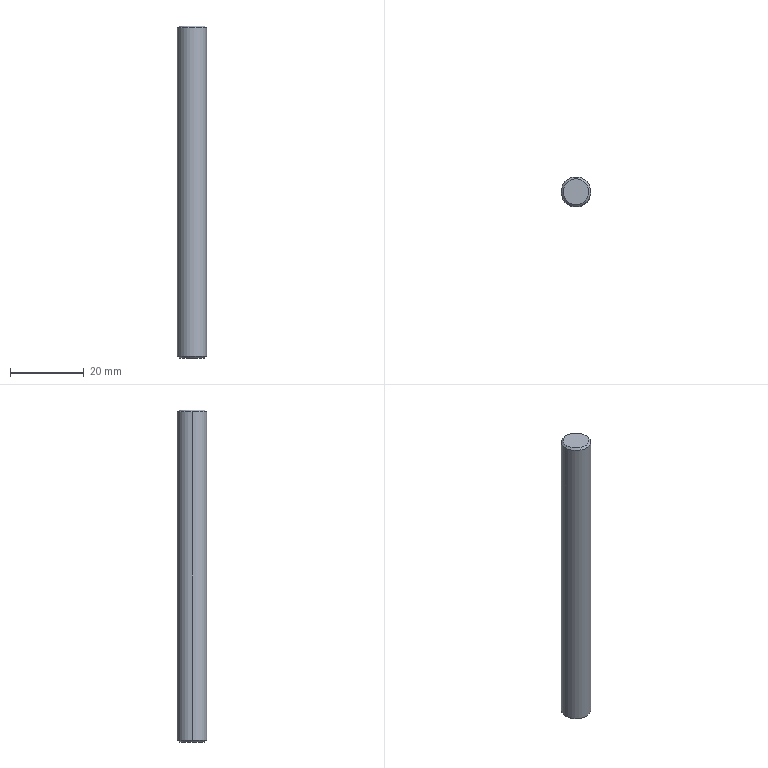Part | STEP file | BCC3 H14_5 | 1 solid | 8 faces | box 8 x 8 x 90 mm | volume 4518 mm3 | cone 4 | cylinder 2 | plane 2 | commonest cylinder face diameters 8 x2
STEP:
#1=CARTESIAN_POINT('',(0.,0.,0.));
#2=DIRECTION('',(0.,0.,1.));
#3=DIRECTION('',(1.,0.,0.));
#4=AXIS2_PLACEMENT_3D('',#1,#2,#3);
#5=CARTESIAN_POINT('',(3.5,0.,45.));
#6=VERTEX_POINT('',#5);
#7=CARTESIAN_POINT('',(-3.5,0.,45.));
#8=VERTEX_POINT('',#7);
#9=CARTESIAN_POINT('',(0.,0.,45.));
#10=DIRECTION('',(0.,0.,1.));
#11=DIRECTION('',(1.,0.,0.));
#12=AXIS2_PLACEMENT_3D('',#9,#10,#11);
#13=CIRCLE('',#12,3.5);
#14=CARTESIAN_POINT('',(0.,0.,45.));
#15=DIRECTION('',(0.,0.,-1.));
#16=DIRECTION('',(-1.,0.,0.));
#17=AXIS2_PLACEMENT_3D('',#14,#15,#16);
#18=CONICAL_SURFACE('',#17,3.5,0.7854);
#19=CARTESIAN_POINT('',(3.142,0.));
#20=DIRECTION('',(-1.,0.));
#21=VECTOR('',#20,1.);
#22=LINE('',#19,#21);
#23=(GEOMETRIC_REPRESENTATION_CONTEXT(2)PARAMETRIC_REPRESENTATION_CONTEXT()REPRESENTATION_CONTEXT('',''));
#24=DEFINITIONAL_REPRESENTATION('',(#22),#23);
#25=PCURVE('',#18,#24);
#26=CARTESIAN_POINT('',(0.,0.,45.));
#27=DIRECTION('',(0.,0.,1.));
#28=DIRECTION('',(1.,0.,0.));
#29=AXIS2_PLACEMENT_3D('',#26,#27,#28);
#30=PLANE('',#29);
#31=CARTESIAN_POINT('',(0.,0.));
#32=DIRECTION('',(1.,0.));
#33=AXIS2_PLACEMENT_2D('',#31,#32);
#34=CIRCLE('',#33,3.5);
#35=(GEOMETRIC_REPRESENTATION_CONTEXT(2)PARAMETRIC_REPRESENTATION_CONTEXT()REPRESENTATION_CONTEXT('',''));
#36=DEFINITIONAL_REPRESENTATION('',(#34),#35);
#37=PCURVE('',#30,#36);
#38=SURFACE_CURVE('',#13,(#25,#37),.PCURVE_S1.);
#39=EDGE_CURVE('',#6,#8,#38,.T.);
#40=ORIENTED_EDGE('',*,*,#39,.F.);
#41=CARTESIAN_POINT('',(4.,0.,44.5));
#42=VERTEX_POINT('',#41);
#43=CARTESIAN_POINT('',(3.5,0.,45.));
#44=DIRECTION('',(0.7071,0.,-0.7071));
#45=VECTOR('',#44,1.);
#46=LINE('',#43,#45);
#47=CARTESIAN_POINT('',(3.142,0.));
#48=DIRECTION('',(0.,1.));
#49=VECTOR('',#48,1.);
#50=LINE('',#47,#49);
#51=(GEOMETRIC_REPRESENTATION_CONTEXT(2)PARAMETRIC_REPRESENTATION_CONTEXT()REPRESENTATION_CONTEXT('',''));
#52=DEFINITIONAL_REPRESENTATION('',(#50),#51);
#53=PCURVE('',#18,#52);
#54=CARTESIAN_POINT('',(0.,0.,45.));
#55=DIRECTION('',(0.,0.,-1.));
#56=DIRECTION('',(-1.,0.,0.));
#57=AXIS2_PLACEMENT_3D('',#54,#55,#56);
#58=CONICAL_SURFACE('',#57,3.5,0.7854);
#59=CARTESIAN_POINT('',(3.142,0.));
#60=DIRECTION('',(0.,1.));
#61=VECTOR('',#60,1.);
#62=LINE('',#59,#61);
#63=(GEOMETRIC_REPRESENTATION_CONTEXT(2)PARAMETRIC_REPRESENTATION_CONTEXT()REPRESENTATION_CONTEXT('',''));
#64=DEFINITIONAL_REPRESENTATION('',(#62),#63);
#65=PCURVE('',#58,#64);
#66=SURFACE_CURVE('',#46,(#53,#65),.PCURVE_S1.);
#67=EDGE_CURVE('',#6,#42,#66,.T.);
#68=ORIENTED_EDGE('',*,*,#67,.T.);
#69=CARTESIAN_POINT('',(-4.,0.,44.5));
#70=VERTEX_POINT('',#69);
#71=CARTESIAN_POINT('',(0.,0.,44.5));
#72=DIRECTION('',(0.,0.,-1.));
#73=DIRECTION('',(1.,0.,0.));
#74=AXIS2_PLACEMENT_3D('',#71,#72,#73);
#75=CIRCLE('',#74,4.);
#76=CARTESIAN_POINT('',(-3.142,0.5));
#77=DIRECTION('',(1.,0.));
#78=VECTOR('',#77,1.);
#79=LINE('',#76,#78);
#80=(GEOMETRIC_REPRESENTATION_CONTEXT(2)PARAMETRIC_REPRESENTATION_CONTEXT()REPRESENTATION_CONTEXT('',''));
#81=DEFINITIONAL_REPRESENTATION('',(#79),#80);
#82=PCURVE('',#18,#81);
#83=CARTESIAN_POINT('',(0.,0.,45.));
#84=DIRECTION('',(0.,0.,-1.));
#85=DIRECTION('',(-1.,0.,0.));
#86=AXIS2_PLACEMENT_3D('',#83,#84,#85);
#87=CYLINDRICAL_SURFACE('',#86,4.);
#88=CARTESIAN_POINT('',(-3.142,0.5));
#89=DIRECTION('',(1.,0.));
#90=VECTOR('',#89,1.);
#91=LINE('',#88,#90);
#92=(GEOMETRIC_REPRESENTATION_CONTEXT(2)PARAMETRIC_REPRESENTATION_CONTEXT()REPRESENTATION_CONTEXT('',''));
#93=DEFINITIONAL_REPRESENTATION('',(#91),#92);
#94=PCURVE('',#87,#93);
#95=SURFACE_CURVE('',#75,(#82,#94),.PCURVE_S1.);
#96=EDGE_CURVE('',#70,#42,#95,.T.);
#97=ORIENTED_EDGE('',*,*,#96,.F.);
#98=CARTESIAN_POINT('',(-3.5,0.,45.));
#99=DIRECTION('',(-0.7071,0.,-0.7071));
#100=VECTOR('',#99,1.);
#101=LINE('',#98,#100);
#102=CARTESIAN_POINT('',(0.,0.));
#103=DIRECTION('',(0.,1.));
#104=VECTOR('',#103,1.);
#105=LINE('',#102,#104);
#106=(GEOMETRIC_REPRESENTATION_CONTEXT(2)PARAMETRIC_REPRESENTATION_CONTEXT()REPRESENTATION_CONTEXT('',''));
#107=DEFINITIONAL_REPRESENTATION('',(#105),#106);
#108=PCURVE('',#18,#107);
#109=CARTESIAN_POINT('',(6.283,0.));
#110=DIRECTION('',(0.,1.));
#111=VECTOR('',#110,1.);
#112=LINE('',#109,#111);
#113=(GEOMETRIC_REPRESENTATION_CONTEXT(2)PARAMETRIC_REPRESENTATION_CONTEXT()REPRESENTATION_CONTEXT('',''));
#114=DEFINITIONAL_REPRESENTATION('',(#112),#113);
#115=PCURVE('',#58,#114);
#116=SURFACE_CURVE('',#101,(#108,#115),.PCURVE_S1.);
#117=EDGE_CURVE('',#8,#70,#116,.T.);
#118=ORIENTED_EDGE('',*,*,#117,.F.);
#119=EDGE_LOOP('',(#40,#68,#97,#118));
#120=FACE_BOUND('',#119,.T.);
#121=ADVANCED_FACE('',(#120),#18,.T.);
#122=CARTESIAN_POINT('',(-3.5,0.,-45.));
#123=VERTEX_POINT('',#122);
#124=CARTESIAN_POINT('',(3.5,0.,-45.));
#125=VERTEX_POINT('',#124);
#126=CARTESIAN_POINT('',(0.,0.,-45.));
#127=DIRECTION('',(0.,0.,-1.));
#128=DIRECTION('',(1.,0.,0.));
#129=AXIS2_PLACEMENT_3D('',#126,#127,#128);
#130=CIRCLE('',#129,3.5);
#131=CARTESIAN_POINT('',(0.,0.,-44.5));
#132=DIRECTION('',(0.,0.,1.));
#133=DIRECTION('',(1.,0.,0.));
#134=AXIS2_PLACEMENT_3D('',#131,#132,#133);
#135=CONICAL_SURFACE('',#134,4.,0.7854);
#136=CARTESIAN_POINT('',(6.283,-0.5));
#137=DIRECTION('',(-1.,0.));
#138=VECTOR('',#137,1.);
#139=LINE('',#136,#138);
#140=(GEOMETRIC_REPRESENTATION_CONTEXT(2)PARAMETRIC_REPRESENTATION_CONTEXT()REPRESENTATION_CONTEXT('',''));
#141=DEFINITIONAL_REPRESENTATION('',(#139),#140);
#142=PCURVE('',#135,#141);
#143=CARTESIAN_POINT('',(0.,0.,-45.));
#144=DIRECTION('',(0.,0.,1.));
#145=DIRECTION('',(1.,0.,0.));
#146=AXIS2_PLACEMENT_3D('',#143,#144,#145);
#147=PLANE('',#146);
#148=CARTESIAN_POINT('',(3.5,0.));
#149=CARTESIAN_POINT('',(3.5,-6.062));
#150=CARTESIAN_POINT('',(-1.75,-3.031));
#151=CARTESIAN_POINT('',(-7.,0.));
#152=CARTESIAN_POINT('',(-1.75,3.031));
#153=CARTESIAN_POINT('',(3.5,6.062));
#154=CARTESIAN_POINT('',(3.5,0.));
#155=(BOUNDED_CURVE()B_SPLINE_CURVE(2,(#148,#149,#150,#151,#152,#153,#154),.UNSPECIFIED.,.T.,.F.)B_SPLINE_CURVE_WITH_KNOTS((1,2,2,2,2,1),(-2.094,0.,2.094,4.189,6.283,8.378),.UNSPECIFIED.)CURVE()GEOMETRIC_REPRESENTATION_ITEM()RATIONAL_B_SPLINE_CURVE((1.,0.5,1.,0.5,1.,0.5,1.))REPRESENTATION_ITEM(''));
#156=(GEOMETRIC_REPRESENTATION_CONTEXT(2)PARAMETRIC_REPRESENTATION_CONTEXT()REPRESENTATION_CONTEXT('',''));
#157=DEFINITIONAL_REPRESENTATION('',(#155),#156);
#158=PCURVE('',#147,#157);
#159=SURFACE_CURVE('',#130,(#142,#158),.PCURVE_S1.);
#160=EDGE_CURVE('',#123,#125,#159,.T.);
#161=ORIENTED_EDGE('',*,*,#160,.F.);
#162=CARTESIAN_POINT('',(-4.,0.,-44.5));
#163=VERTEX_POINT('',#162);
#164=CARTESIAN_POINT('',(-4.,0.,-44.5));
#165=DIRECTION('',(-0.7071,0.,0.7071));
#166=VECTOR('',#165,1.);
#167=LINE('',#164,#166);
#168=CARTESIAN_POINT('',(3.142,0.));
#169=DIRECTION('',(0.,1.));
#170=VECTOR('',#169,1.);
#171=LINE('',#168,#170);
#172=(GEOMETRIC_REPRESENTATION_CONTEXT(2)PARAMETRIC_REPRESENTATION_CONTEXT()REPRESENTATION_CONTEXT('',''));
#173=DEFINITIONAL_REPRESENTATION('',(#171),#172);
#174=PCURVE('',#135,#173);
#175=CARTESIAN_POINT('',(0.,0.,-44.5));
#176=DIRECTION('',(0.,0.,1.));
#177=DIRECTION('',(1.,0.,0.));
#178=AXIS2_PLACEMENT_3D('',#175,#176,#177);
#179=CONICAL_SURFACE('',#178,4.,0.7854);
#180=CARTESIAN_POINT('',(3.142,0.));
#181=DIRECTION('',(0.,1.));
#182=VECTOR('',#181,1.);
#183=LINE('',#180,#182);
#184=(GEOMETRIC_REPRESENTATION_CONTEXT(2)PARAMETRIC_REPRESENTATION_CONTEXT()REPRESENTATION_CONTEXT('',''));
#185=DEFINITIONAL_REPRESENTATION('',(#183),#184);
#186=PCURVE('',#179,#185);
#187=SURFACE_CURVE('',#167,(#174,#186),.PCURVE_S1.);
#188=EDGE_CURVE('',#123,#163,#187,.T.);
#189=ORIENTED_EDGE('',*,*,#188,.T.);
#190=CARTESIAN_POINT('',(4.,0.,-44.5));
#191=VERTEX_POINT('',#190);
#192=CARTESIAN_POINT('',(0.,0.,-44.5));
#193=DIRECTION('',(0.,0.,1.));
#194=DIRECTION('',(1.,0.,0.));
#195=AXIS2_PLACEMENT_3D('',#192,#193,#194);
#196=CIRCLE('',#195,4.);
#197=CARTESIAN_POINT('',(0.,0.));
#198=DIRECTION('',(1.,0.));
#199=VECTOR('',#198,1.);
#200=LINE('',#197,#199);
#201=(GEOMETRIC_REPRESENTATION_CONTEXT(2)PARAMETRIC_REPRESENTATION_CONTEXT()REPRESENTATION_CONTEXT('',''));
#202=DEFINITIONAL_REPRESENTATION('',(#200),#201);
#203=PCURVE('',#135,#202);
#204=CARTESIAN_POINT('',(3.142,89.5));
#205=DIRECTION('',(-1.,0.));
#206=VECTOR('',#205,1.);
#207=LINE('',#204,#206);
#208=(GEOMETRIC_REPRESENTATION_CONTEXT(2)PARAMETRIC_REPRESENTATION_CONTEXT()REPRESENTATION_CONTEXT('',''));
#209=DEFINITIONAL_REPRESENTATION('',(#207),#208);
#210=PCURVE('',#87,#209);
#211=SURFACE_CURVE('',#196,(#203,#210),.PCURVE_S1.);
#212=EDGE_CURVE('',#191,#163,#211,.T.);
#213=ORIENTED_EDGE('',*,*,#212,.F.);
#214=CARTESIAN_POINT('',(4.,0.,-44.5));
#215=DIRECTION('',(0.7071,0.,0.7071));
#216=VECTOR('',#215,1.);
#217=LINE('',#214,#216);
#218=CARTESIAN_POINT('',(0.,0.));
#219=DIRECTION('',(0.,1.));
#220=VECTOR('',#219,1.);
#221=LINE('',#218,#220);
#222=(GEOMETRIC_REPRESENTATION_CONTEXT(2)PARAMETRIC_REPRESENTATION_CONTEXT()REPRESENTATION_CONTEXT('',''));
#223=DEFINITIONAL_REPRESENTATION('',(#221),#222);
#224=PCURVE('',#135,#223);
#225=CARTESIAN_POINT('',(6.283,0.));
#226=DIRECTION('',(0.,1.));
#227=VECTOR('',#226,1.);
#228=LINE('',#225,#227);
#229=(GEOMETRIC_REPRESENTATION_CONTEXT(2)PARAMETRIC_REPRESENTATION_CONTEXT()REPRESENTATION_CONTEXT('',''));
#230=DEFINITIONAL_REPRESENTATION('',(#228),#229);
#231=PCURVE('',#179,#230);
#232=SURFACE_CURVE('',#217,(#224,#231),.PCURVE_S1.);
#233=EDGE_CURVE('',#125,#191,#232,.T.);
#234=ORIENTED_EDGE('',*,*,#233,.F.);
#235=EDGE_LOOP('',(#161,#189,#213,#234));
#236=FACE_BOUND('',#235,.T.);
#237=ADVANCED_FACE('',(#236),#135,.T.);
#238=ORIENTED_EDGE('',*,*,#96,.T.);
#239=CARTESIAN_POINT('',(4.,0.,45.));
#240=DIRECTION('',(0.,0.,-1.));
#241=VECTOR('',#240,1.);
#242=LINE('',#239,#241);
#243=CARTESIAN_POINT('',(3.142,0.));
#244=DIRECTION('',(0.,1.));
#245=VECTOR('',#244,1.);
#246=LINE('',#243,#245);
#247=(GEOMETRIC_REPRESENTATION_CONTEXT(2)PARAMETRIC_REPRESENTATION_CONTEXT()REPRESENTATION_CONTEXT('',''));
#248=DEFINITIONAL_REPRESENTATION('',(#246),#247);
#249=PCURVE('',#87,#248);
#250=CARTESIAN_POINT('',(0.,0.,45.));
#251=DIRECTION('',(0.,0.,-1.));
#252=DIRECTION('',(-1.,0.,0.));
#253=AXIS2_PLACEMENT_3D('',#250,#251,#252);
#254=CYLINDRICAL_SURFACE('',#253,4.);
#255=CARTESIAN_POINT('',(3.142,0.));
#256=DIRECTION('',(0.,1.));
#257=VECTOR('',#256,1.);
#258=LINE('',#255,#257);
#259=(GEOMETRIC_REPRESENTATION_CONTEXT(2)PARAMETRIC_REPRESENTATION_CONTEXT()REPRESENTATION_CONTEXT('',''));
#260=DEFINITIONAL_REPRESENTATION('',(#258),#259);
#261=PCURVE('',#254,#260);
#262=SURFACE_CURVE('',#242,(#249,#261),.PCURVE_S1.);
#263=EDGE_CURVE('',#42,#191,#262,.T.);
#264=ORIENTED_EDGE('',*,*,#263,.T.);
#265=ORIENTED_EDGE('',*,*,#212,.T.);
#266=CARTESIAN_POINT('',(-4.,0.,45.));
#267=DIRECTION('',(0.,0.,-1.));
#268=VECTOR('',#267,1.);
#269=LINE('',#266,#268);
#270=CARTESIAN_POINT('',(0.,0.));
#271=DIRECTION('',(0.,1.));
#272=VECTOR('',#271,1.);
#273=LINE('',#270,#272);
#274=(GEOMETRIC_REPRESENTATION_CONTEXT(2)PARAMETRIC_REPRESENTATION_CONTEXT()REPRESENTATION_CONTEXT('',''));
#275=DEFINITIONAL_REPRESENTATION('',(#273),#274);
#276=PCURVE('',#87,#275);
#277=CARTESIAN_POINT('',(6.283,0.));
#278=DIRECTION('',(0.,1.));
#279=VECTOR('',#278,1.);
#280=LINE('',#277,#279);
#281=(GEOMETRIC_REPRESENTATION_CONTEXT(2)PARAMETRIC_REPRESENTATION_CONTEXT()REPRESENTATION_CONTEXT('',''));
#282=DEFINITIONAL_REPRESENTATION('',(#280),#281);
#283=PCURVE('',#254,#282);
#284=SURFACE_CURVE('',#269,(#276,#283),.PCURVE_S1.);
#285=EDGE_CURVE('',#70,#163,#284,.T.);
#286=ORIENTED_EDGE('',*,*,#285,.F.);
#287=EDGE_LOOP('',(#238,#264,#265,#286));
#288=FACE_BOUND('',#287,.T.);
#289=ADVANCED_FACE('',(#288),#87,.T.);
#290=ORIENTED_EDGE('',*,*,#263,.F.);
#291=CARTESIAN_POINT('',(0.,0.,44.5));
#292=DIRECTION('',(0.,0.,-1.));
#293=DIRECTION('',(1.,0.,0.));
#294=AXIS2_PLACEMENT_3D('',#291,#292,#293);
#295=CIRCLE('',#294,4.);
#296=CARTESIAN_POINT('',(3.142,0.5));
#297=DIRECTION('',(1.,0.));
#298=VECTOR('',#297,1.);
#299=LINE('',#296,#298);
#300=(GEOMETRIC_REPRESENTATION_CONTEXT(2)PARAMETRIC_REPRESENTATION_CONTEXT()REPRESENTATION_CONTEXT('',''));
#301=DEFINITIONAL_REPRESENTATION('',(#299),#300);
#302=PCURVE('',#254,#301);
#303=CARTESIAN_POINT('',(3.142,0.5));
#304=DIRECTION('',(1.,0.));
#305=VECTOR('',#304,1.);
#306=LINE('',#303,#305);
#307=(GEOMETRIC_REPRESENTATION_CONTEXT(2)PARAMETRIC_REPRESENTATION_CONTEXT()REPRESENTATION_CONTEXT('',''));
#308=DEFINITIONAL_REPRESENTATION('',(#306),#307);
#309=PCURVE('',#58,#308);
#310=SURFACE_CURVE('',#295,(#302,#309),.PCURVE_S1.);
#311=EDGE_CURVE('',#42,#70,#310,.T.);
#312=ORIENTED_EDGE('',*,*,#311,.T.);
#313=ORIENTED_EDGE('',*,*,#285,.T.);
#314=CARTESIAN_POINT('',(0.,0.,-44.5));
#315=DIRECTION('',(0.,0.,1.));
#316=DIRECTION('',(1.,0.,0.));
#317=AXIS2_PLACEMENT_3D('',#314,#315,#316);
#318=CIRCLE('',#317,4.);
#319=CARTESIAN_POINT('',(9.425,89.5));
#320=DIRECTION('',(-1.,0.));
#321=VECTOR('',#320,1.);
#322=LINE('',#319,#321);
#323=(GEOMETRIC_REPRESENTATION_CONTEXT(2)PARAMETRIC_REPRESENTATION_CONTEXT()REPRESENTATION_CONTEXT('',''));
#324=DEFINITIONAL_REPRESENTATION('',(#322),#323);
#325=PCURVE('',#254,#324);
#326=CARTESIAN_POINT('',(0.,0.));
#327=DIRECTION('',(1.,0.));
#328=VECTOR('',#327,1.);
#329=LINE('',#326,#328);
#330=(GEOMETRIC_REPRESENTATION_CONTEXT(2)PARAMETRIC_REPRESENTATION_CONTEXT()REPRESENTATION_CONTEXT('',''));
#331=DEFINITIONAL_REPRESENTATION('',(#329),#330);
#332=PCURVE('',#179,#331);
#333=SURFACE_CURVE('',#318,(#325,#332),.PCURVE_S1.);
#334=EDGE_CURVE('',#163,#191,#333,.T.);
#335=ORIENTED_EDGE('',*,*,#334,.T.);
#336=EDGE_LOOP('',(#290,#312,#313,#335));
#337=FACE_BOUND('',#336,.T.);
#338=ADVANCED_FACE('',(#337),#254,.T.);
#339=CARTESIAN_POINT('',(0.,0.,45.));
#340=DIRECTION('',(0.,0.,1.));
#341=DIRECTION('',(1.,0.,0.));
#342=AXIS2_PLACEMENT_3D('',#339,#340,#341);
#343=CIRCLE('',#342,3.5);
#344=CARTESIAN_POINT('',(0.,0.));
#345=DIRECTION('',(1.,0.));
#346=AXIS2_PLACEMENT_2D('',#344,#345);
#347=CIRCLE('',#346,3.5);
#348=(GEOMETRIC_REPRESENTATION_CONTEXT(2)PARAMETRIC_REPRESENTATION_CONTEXT()REPRESENTATION_CONTEXT('',''));
#349=DEFINITIONAL_REPRESENTATION('',(#347),#348);
#350=PCURVE('',#30,#349);
#351=CARTESIAN_POINT('',(9.425,0.));
#352=DIRECTION('',(-1.,0.));
#353=VECTOR('',#352,1.);
#354=LINE('',#351,#353);
#355=(GEOMETRIC_REPRESENTATION_CONTEXT(2)PARAMETRIC_REPRESENTATION_CONTEXT()REPRESENTATION_CONTEXT('',''));
#356=DEFINITIONAL_REPRESENTATION('',(#354),#355);
#357=PCURVE('',#58,#356);
#358=SURFACE_CURVE('',#343,(#350,#357),.PCURVE_S1.);
#359=EDGE_CURVE('',#8,#6,#358,.T.);
#360=ORIENTED_EDGE('',*,*,#359,.T.);
#361=ORIENTED_EDGE('',*,*,#39,.T.);
#362=EDGE_LOOP('',(#360,#361));
#363=FACE_BOUND('',#362,.T.);
#364=ADVANCED_FACE('',(#363),#30,.T.);
#365=CARTESIAN_POINT('',(0.,0.,-45.));
#366=DIRECTION('',(0.,0.,-1.));
#367=DIRECTION('',(1.,0.,0.));
#368=AXIS2_PLACEMENT_3D('',#365,#366,#367);
#369=CIRCLE('',#368,3.5);
#370=CARTESIAN_POINT('',(3.5,0.));
#371=CARTESIAN_POINT('',(3.5,-6.062));
#372=CARTESIAN_POINT('',(-1.75,-3.031));
#373=CARTESIAN_POINT('',(-7.,0.));
#374=CARTESIAN_POINT('',(-1.75,3.031));
#375=CARTESIAN_POINT('',(3.5,6.062));
#376=CARTESIAN_POINT('',(3.5,0.));
#377=(BOUNDED_CURVE()B_SPLINE_CURVE(2,(#370,#371,#372,#373,#374,#375,#376),.UNSPECIFIED.,.T.,.F.)B_SPLINE_CURVE_WITH_KNOTS((1,2,2,2,2,1),(-2.094,0.,2.094,4.189,6.283,8.378),.UNSPECIFIED.)CURVE()GEOMETRIC_REPRESENTATION_ITEM()RATIONAL_B_SPLINE_CURVE((1.,0.5,1.,0.5,1.,0.5,1.))REPRESENTATION_ITEM(''));
#378=(GEOMETRIC_REPRESENTATION_CONTEXT(2)PARAMETRIC_REPRESENTATION_CONTEXT()REPRESENTATION_CONTEXT('',''));
#379=DEFINITIONAL_REPRESENTATION('',(#377),#378);
#380=PCURVE('',#147,#379);
#381=CARTESIAN_POINT('',(6.283,-0.5));
#382=DIRECTION('',(-1.,0.));
#383=VECTOR('',#382,1.);
#384=LINE('',#381,#383);
#385=(GEOMETRIC_REPRESENTATION_CONTEXT(2)PARAMETRIC_REPRESENTATION_CONTEXT()REPRESENTATION_CONTEXT('',''));
#386=DEFINITIONAL_REPRESENTATION('',(#384),#385);
#387=PCURVE('',#179,#386);
#388=SURFACE_CURVE('',#369,(#380,#387),.PCURVE_S1.);
#389=EDGE_CURVE('',#125,#123,#388,.T.);
#390=ORIENTED_EDGE('',*,*,#389,.T.);
#391=ORIENTED_EDGE('',*,*,#160,.T.);
#392=EDGE_LOOP('',(#390,#391));
#393=FACE_BOUND('',#392,.T.);
#394=ADVANCED_FACE('',(#393),#147,.F.);
#395=ORIENTED_EDGE('',*,*,#188,.F.);
#396=ORIENTED_EDGE('',*,*,#389,.F.);
#397=ORIENTED_EDGE('',*,*,#233,.T.);
#398=ORIENTED_EDGE('',*,*,#334,.F.);
#399=EDGE_LOOP('',(#395,#396,#397,#398));
#400=FACE_BOUND('',#399,.T.);
#401=ADVANCED_FACE('',(#400),#179,.T.);
#402=ORIENTED_EDGE('',*,*,#67,.F.);
#403=ORIENTED_EDGE('',*,*,#359,.F.);
#404=ORIENTED_EDGE('',*,*,#117,.T.);
#405=ORIENTED_EDGE('',*,*,#311,.F.);
#406=EDGE_LOOP('',(#402,#403,#404,#405));
#407=FACE_BOUND('',#406,.T.);
#408=ADVANCED_FACE('',(#407),#58,.T.);
#409=CLOSED_SHELL('',(#121,#237,#289,#338,#364,#394,#401,#408));
#410=MANIFOLD_SOLID_BREP('',#409);
#411=(LENGTH_UNIT()NAMED_UNIT(*)SI_UNIT(.MILLI.,.METRE.));
#412=UNCERTAINTY_MEASURE_WITH_UNIT(LENGTH_MEASURE(0.0000001),#411,'','');
#413=(NAMED_UNIT(*)PLANE_ANGLE_UNIT()SI_UNIT($,.RADIAN.));
#414=(NAMED_UNIT(*)SI_UNIT($,.STERADIAN.)SOLID_ANGLE_UNIT());
#415=(GEOMETRIC_REPRESENTATION_CONTEXT(3)GLOBAL_UNCERTAINTY_ASSIGNED_CONTEXT((#412))GLOBAL_UNIT_ASSIGNED_CONTEXT((#411,#413,#414))REPRESENTATION_CONTEXT('',''));
#416=ADVANCED_BREP_SHAPE_REPRESENTATION('',(#4,#410),#415);